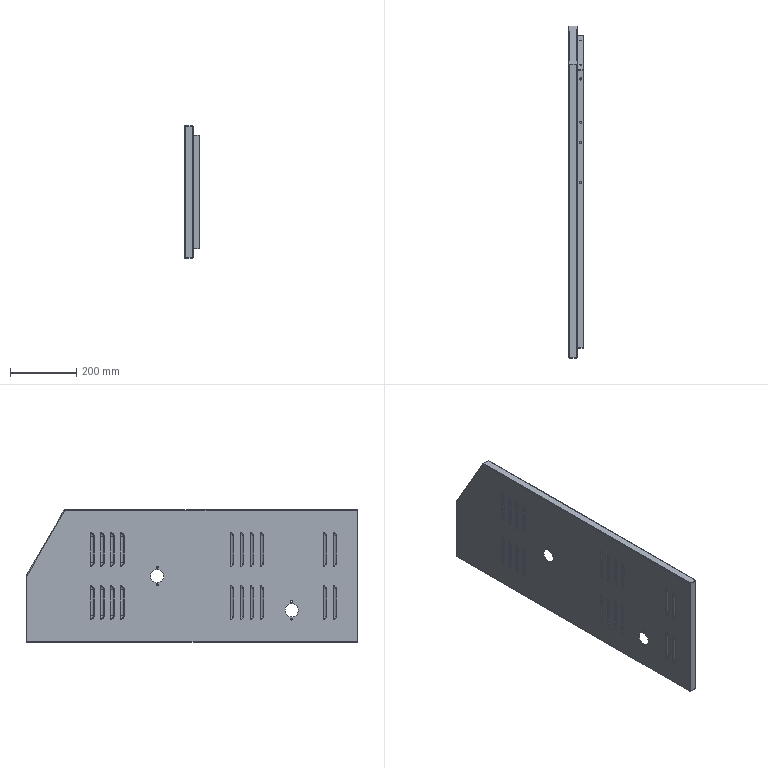Part | SolidWorks | features Cut 4, EdgeFlange 3, FormToolInstance 3, ICE 2, FlatPattern 1, Fold 1, SMBaseFlange 1, SheetMetal 1, UnFold 1 | 1 solid | 541 faces | box 43.8 x 1000 x 400 mm | volume 681227 mm3 | torus 160 | cylinder 144 | plane 137 | spline 100 | commonest cylinder face diameters 6 x28 3.6 x20 29 x20 31.4 x20 6.5 x16 2 x15